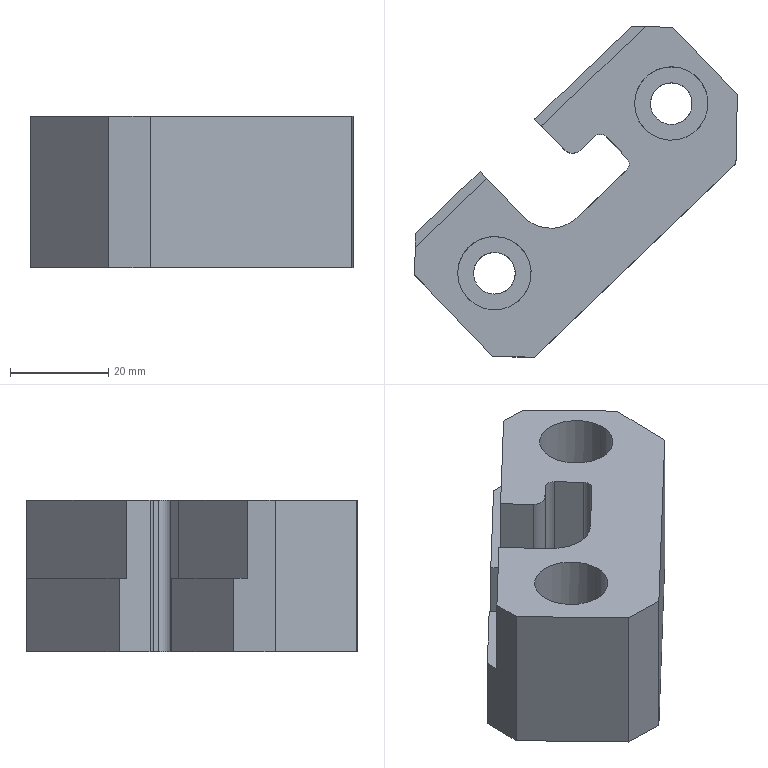Part | STEP file | gslz 2016.10.28-13_id1666_x_t | 1 solid | 34 faces | box 65.839 x 67.482 x 31 mm | volume 54828 mm3 | plane 24 | cylinder 10 | commonest cylinder face diameters 3.5 x2 8.5 x2 10 x2 15 x2 4.5 x1 15.5 x1